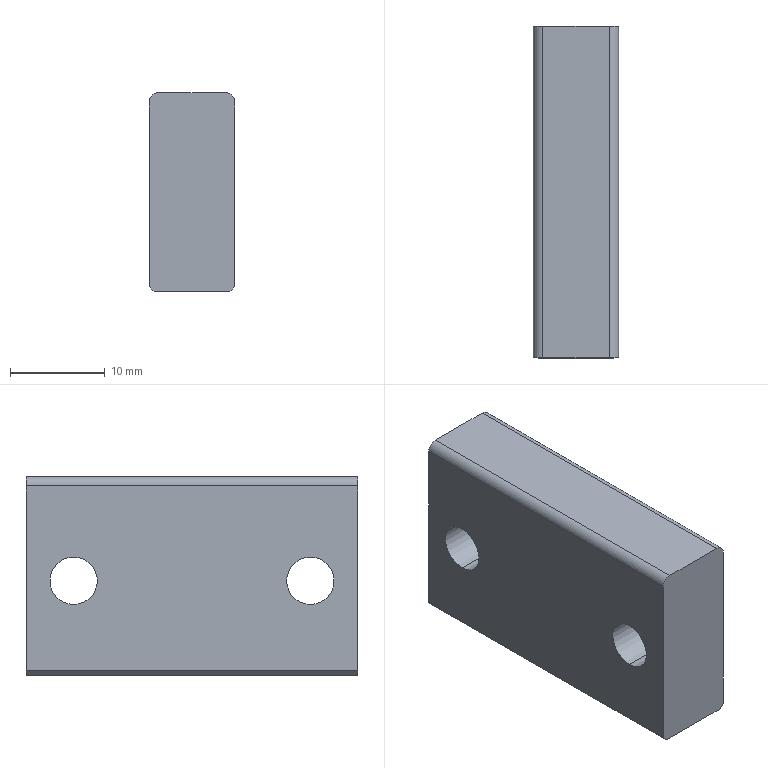Part | SolidWorks | features HoleWzd 2, Chamfer 1, Extrusion 1, Fillet 1 | 1 solid | 22 faces | box 9 x 35 x 21 mm | volume 5976 mm3 | cylinder 10 | plane 8 | cone 4 | commonest cylinder face diameters 3.3 x4 5 x4 2 x2
STEP:
#1=CARTESIAN_POINT('',(6.15,4.5,15.));
#2=VERTEX_POINT('',#1);
#3=CARTESIAN_POINT('',(2.85,4.5,15.));
#4=VERTEX_POINT('',#3);
#5=CARTESIAN_POINT('',(4.5,4.5,15.));
#6=DIRECTION('',(0.,0.,-1.));
#7=DIRECTION('',(-1.,0.,0.));
#8=AXIS2_PLACEMENT_3D('',#5,#6,#7);
#9=CIRCLE('',#8,1.65);
#10=EDGE_CURVE('',#2,#4,#9,.T.);
#11=ORIENTED_EDGE('',*,*,#10,.F.);
#12=CARTESIAN_POINT('',(6.15,4.5,0.));
#13=VERTEX_POINT('',#12);
#14=CARTESIAN_POINT('',(6.15,4.5,0.));
#15=DIRECTION('',(0.,0.,-1.));
#16=VECTOR('',#15,1000.);
#17=LINE('',#14,#16);
#18=EDGE_CURVE('',#2,#13,#17,.T.);
#19=ORIENTED_EDGE('',*,*,#18,.T.);
#20=CARTESIAN_POINT('',(2.85,4.5,0.));
#21=VERTEX_POINT('',#20);
#22=CARTESIAN_POINT('',(4.5,4.5,0.));
#23=DIRECTION('',(0.,0.,-1.));
#24=DIRECTION('',(-1.,0.,0.));
#25=AXIS2_PLACEMENT_3D('',#22,#23,#24);
#26=CIRCLE('',#25,1.65);
#27=EDGE_CURVE('',#13,#21,#26,.T.);
#28=ORIENTED_EDGE('',*,*,#27,.T.);
#29=CARTESIAN_POINT('',(2.85,4.5,0.));
#30=DIRECTION('',(0.,0.,-1.));
#31=VECTOR('',#30,1000.);
#32=LINE('',#29,#31);
#33=EDGE_CURVE('',#4,#21,#32,.T.);
#34=ORIENTED_EDGE('',*,*,#33,.F.);
#35=EDGE_LOOP('',(#11,#19,#28,#34));
#36=FACE_OUTER_BOUND('',#35,.T.);
#37=CARTESIAN_POINT('',(4.5,4.5,0.));
#38=DIRECTION('',(0.,0.,-1.));
#39=DIRECTION('',(-1.,0.,0.));
#40=AXIS2_PLACEMENT_3D('',#37,#38,#39);
#41=CYLINDRICAL_SURFACE('',#40,1.65);
#42=ADVANCED_FACE('',(#36),#41,.F.);
#43=CARTESIAN_POINT('',(4.5,4.5,15.991));
#44=VERTEX_POINT('',#43);
#45=CARTESIAN_POINT('',(2.85,4.5,15.));
#46=DIRECTION('',(-0.8572,0.,-0.515));
#47=VECTOR('',#46,1000.);
#48=LINE('',#45,#47);
#49=EDGE_CURVE('',#44,#4,#48,.T.);
#50=ORIENTED_EDGE('',*,*,#49,.F.);
#51=CARTESIAN_POINT('',(6.15,4.5,15.));
#52=DIRECTION('',(0.8572,0.,-0.515));
#53=VECTOR('',#52,1000.);
#54=LINE('',#51,#53);
#55=EDGE_CURVE('',#44,#2,#54,.T.);
#56=ORIENTED_EDGE('',*,*,#55,.T.);
#57=ORIENTED_EDGE('',*,*,#10,.T.);
#58=EDGE_LOOP('',(#50,#56,#57));
#59=FACE_OUTER_BOUND('',#58,.T.);
#60=CARTESIAN_POINT('',(4.5,4.5,15.));
#61=DIRECTION('',(0.,0.,-1.));
#62=DIRECTION('',(-1.,0.,0.));
#63=AXIS2_PLACEMENT_3D('',#60,#61,#62);
#64=CONICAL_SURFACE('',#63,1.65,1.03);
#65=ADVANCED_FACE('',(#59),#64,.F.);
#66=CARTESIAN_POINT('',(6.15,-4.5,15.));
#67=VERTEX_POINT('',#66);
#68=CARTESIAN_POINT('',(2.85,-4.5,15.));
#69=VERTEX_POINT('',#68);
#70=CARTESIAN_POINT('',(4.5,-4.5,15.));
#71=DIRECTION('',(0.,0.,-1.));
#72=DIRECTION('',(-1.,0.,0.));
#73=AXIS2_PLACEMENT_3D('',#70,#71,#72);
#74=CIRCLE('',#73,1.65);
#75=EDGE_CURVE('',#67,#69,#74,.T.);
#76=ORIENTED_EDGE('',*,*,#75,.F.);
#77=CARTESIAN_POINT('',(6.15,-4.5,0.));
#78=VERTEX_POINT('',#77);
#79=CARTESIAN_POINT('',(6.15,-4.5,0.));
#80=DIRECTION('',(0.,0.,-1.));
#81=VECTOR('',#80,1000.);
#82=LINE('',#79,#81);
#83=EDGE_CURVE('',#67,#78,#82,.T.);
#84=ORIENTED_EDGE('',*,*,#83,.T.);
#85=CARTESIAN_POINT('',(2.85,-4.5,0.));
#86=VERTEX_POINT('',#85);
#87=CARTESIAN_POINT('',(4.5,-4.5,0.));
#88=DIRECTION('',(0.,0.,-1.));
#89=DIRECTION('',(-1.,0.,0.));
#90=AXIS2_PLACEMENT_3D('',#87,#88,#89);
#91=CIRCLE('',#90,1.65);
#92=EDGE_CURVE('',#78,#86,#91,.T.);
#93=ORIENTED_EDGE('',*,*,#92,.T.);
#94=CARTESIAN_POINT('',(2.85,-4.5,0.));
#95=DIRECTION('',(0.,0.,-1.));
#96=VECTOR('',#95,1000.);
#97=LINE('',#94,#96);
#98=EDGE_CURVE('',#69,#86,#97,.T.);
#99=ORIENTED_EDGE('',*,*,#98,.F.);
#100=EDGE_LOOP('',(#76,#84,#93,#99));
#101=FACE_OUTER_BOUND('',#100,.T.);
#102=CARTESIAN_POINT('',(4.5,-4.5,0.));
#103=DIRECTION('',(0.,0.,-1.));
#104=DIRECTION('',(-1.,0.,0.));
#105=AXIS2_PLACEMENT_3D('',#102,#103,#104);
#106=CYLINDRICAL_SURFACE('',#105,1.65);
#107=ADVANCED_FACE('',(#101),#106,.F.);
#108=CARTESIAN_POINT('',(4.5,-4.5,15.991));
#109=VERTEX_POINT('',#108);
#110=CARTESIAN_POINT('',(2.85,-4.5,15.));
#111=DIRECTION('',(-0.8572,0.,-0.515));
#112=VECTOR('',#111,1000.);
#113=LINE('',#110,#112);
#114=EDGE_CURVE('',#109,#69,#113,.T.);
#115=ORIENTED_EDGE('',*,*,#114,.F.);
#116=CARTESIAN_POINT('',(6.15,-4.5,15.));
#117=DIRECTION('',(0.8572,0.,-0.515));
#118=VECTOR('',#117,1000.);
#119=LINE('',#116,#118);
#120=EDGE_CURVE('',#109,#67,#119,.T.);
#121=ORIENTED_EDGE('',*,*,#120,.T.);
#122=ORIENTED_EDGE('',*,*,#75,.T.);
#123=EDGE_LOOP('',(#115,#121,#122));
#124=FACE_OUTER_BOUND('',#123,.T.);
#125=CARTESIAN_POINT('',(4.5,-4.5,15.));
#126=DIRECTION('',(0.,0.,-1.));
#127=DIRECTION('',(-1.,0.,0.));
#128=AXIS2_PLACEMENT_3D('',#125,#126,#127);
#129=CONICAL_SURFACE('',#128,1.65,1.03);
#130=ADVANCED_FACE('',(#124),#129,.F.);
#131=CARTESIAN_POINT('',(0.,12.5,12.5));
#132=VERTEX_POINT('',#131);
#133=CARTESIAN_POINT('',(0.,12.5,7.5));
#134=VERTEX_POINT('',#133);
#135=CARTESIAN_POINT('',(0.,12.5,10.));
#136=DIRECTION('',(1.,0.,0.));
#137=DIRECTION('',(0.,0.,-1.));
#138=AXIS2_PLACEMENT_3D('',#135,#136,#137);
#139=CIRCLE('',#138,2.5);
#140=EDGE_CURVE('',#132,#134,#139,.T.);
#141=ORIENTED_EDGE('',*,*,#140,.F.);
#142=CARTESIAN_POINT('',(9.,12.5,12.5));
#143=VERTEX_POINT('',#142);
#144=CARTESIAN_POINT('',(9.,12.5,12.5));
#145=DIRECTION('',(1.,0.,0.));
#146=VECTOR('',#145,1000.);
#147=LINE('',#144,#146);
#148=EDGE_CURVE('',#132,#143,#147,.T.);
#149=ORIENTED_EDGE('',*,*,#148,.T.);
#150=CARTESIAN_POINT('',(9.,12.5,7.5));
#151=VERTEX_POINT('',#150);
#152=CARTESIAN_POINT('',(9.,12.5,10.));
#153=DIRECTION('',(1.,0.,0.));
#154=DIRECTION('',(0.,0.,-1.));
#155=AXIS2_PLACEMENT_3D('',#152,#153,#154);
#156=CIRCLE('',#155,2.5);
#157=EDGE_CURVE('',#143,#151,#156,.T.);
#158=ORIENTED_EDGE('',*,*,#157,.T.);
#159=CARTESIAN_POINT('',(9.,12.5,7.5));
#160=DIRECTION('',(1.,0.,0.));
#161=VECTOR('',#160,1000.);
#162=LINE('',#159,#161);
#163=EDGE_CURVE('',#134,#151,#162,.T.);
#164=ORIENTED_EDGE('',*,*,#163,.F.);
#165=EDGE_LOOP('',(#141,#149,#158,#164));
#166=FACE_OUTER_BOUND('',#165,.T.);
#167=CARTESIAN_POINT('',(9.,12.5,10.));
#168=DIRECTION('',(1.,0.,0.));
#169=DIRECTION('',(0.,0.,-1.));
#170=AXIS2_PLACEMENT_3D('',#167,#168,#169);
#171=CYLINDRICAL_SURFACE('',#170,2.5);
#172=ADVANCED_FACE('',(#166),#171,.F.);
#173=CARTESIAN_POINT('',(0.,-12.5,12.5));
#174=VERTEX_POINT('',#173);
#175=CARTESIAN_POINT('',(0.,-12.5,7.5));
#176=VERTEX_POINT('',#175);
#177=CARTESIAN_POINT('',(0.,-12.5,10.));
#178=DIRECTION('',(1.,0.,0.));
#179=DIRECTION('',(0.,0.,-1.));
#180=AXIS2_PLACEMENT_3D('',#177,#178,#179);
#181=CIRCLE('',#180,2.5);
#182=EDGE_CURVE('',#174,#176,#181,.T.);
#183=ORIENTED_EDGE('',*,*,#182,.F.);
#184=CARTESIAN_POINT('',(9.,-12.5,12.5));
#185=VERTEX_POINT('',#184);
#186=CARTESIAN_POINT('',(9.,-12.5,12.5));
#187=DIRECTION('',(1.,0.,0.));
#188=VECTOR('',#187,1000.);
#189=LINE('',#186,#188);
#190=EDGE_CURVE('',#174,#185,#189,.T.);
#191=ORIENTED_EDGE('',*,*,#190,.T.);
#192=CARTESIAN_POINT('',(9.,-12.5,7.5));
#193=VERTEX_POINT('',#192);
#194=CARTESIAN_POINT('',(9.,-12.5,10.));
#195=DIRECTION('',(1.,0.,0.));
#196=DIRECTION('',(0.,0.,-1.));
#197=AXIS2_PLACEMENT_3D('',#194,#195,#196);
#198=CIRCLE('',#197,2.5);
#199=EDGE_CURVE('',#185,#193,#198,.T.);
#200=ORIENTED_EDGE('',*,*,#199,.T.);
#201=CARTESIAN_POINT('',(9.,-12.5,7.5));
#202=DIRECTION('',(1.,0.,0.));
#203=VECTOR('',#202,1000.);
#204=LINE('',#201,#203);
#205=EDGE_CURVE('',#176,#193,#204,.T.);
#206=ORIENTED_EDGE('',*,*,#205,.F.);
#207=EDGE_LOOP('',(#183,#191,#200,#206));
#208=FACE_OUTER_BOUND('',#207,.T.);
#209=CARTESIAN_POINT('',(9.,-12.5,10.));
#210=DIRECTION('',(1.,0.,0.));
#211=DIRECTION('',(0.,0.,-1.));
#212=AXIS2_PLACEMENT_3D('',#209,#210,#211);
#213=CYLINDRICAL_SURFACE('',#212,2.5);
#214=ADVANCED_FACE('',(#208),#213,.F.);
#215=CARTESIAN_POINT('',(0.,12.5,10.));
#216=DIRECTION('',(1.,0.,0.));
#217=DIRECTION('',(0.,0.,-1.));
#218=AXIS2_PLACEMENT_3D('',#215,#216,#217);
#219=CIRCLE('',#218,2.5);
#220=EDGE_CURVE('',#134,#132,#219,.T.);
#221=ORIENTED_EDGE('',*,*,#220,.T.);
#222=ORIENTED_EDGE('',*,*,#140,.T.);
#223=EDGE_LOOP('',(#221,#222));
#224=FACE_BOUND('',#223,.T.);
#225=CARTESIAN_POINT('',(0.,-12.5,10.));
#226=DIRECTION('',(1.,0.,0.));
#227=DIRECTION('',(0.,0.,-1.));
#228=AXIS2_PLACEMENT_3D('',#225,#226,#227);
#229=CIRCLE('',#228,2.5);
#230=EDGE_CURVE('',#176,#174,#229,.T.);
#231=ORIENTED_EDGE('',*,*,#230,.T.);
#232=ORIENTED_EDGE('',*,*,#182,.T.);
#233=EDGE_LOOP('',(#231,#232));
#234=FACE_BOUND('',#233,.T.);
#235=CARTESIAN_POINT('',(0.,17.5,20.));
#236=VERTEX_POINT('',#235);
#237=CARTESIAN_POINT('',(0.,17.5,0.5));
#238=VERTEX_POINT('',#237);
#239=CARTESIAN_POINT('',(0.,17.5,21.));
#240=DIRECTION('',(0.,0.,-1.));
#241=VECTOR('',#240,1000.);
#242=LINE('',#239,#241);
#243=EDGE_CURVE('',#236,#238,#242,.T.);
#244=ORIENTED_EDGE('',*,*,#243,.T.);
#245=CARTESIAN_POINT('',(0.,-17.5,0.5));
#246=VERTEX_POINT('',#245);
#247=CARTESIAN_POINT('',(0.,17.5,0.5));
#248=DIRECTION('',(0.,-1.,0.));
#249=VECTOR('',#248,1000.);
#250=LINE('',#247,#249);
#251=EDGE_CURVE('',#238,#246,#250,.T.);
#252=ORIENTED_EDGE('',*,*,#251,.T.);
#253=CARTESIAN_POINT('',(0.,-17.5,20.));
#254=VERTEX_POINT('',#253);
#255=CARTESIAN_POINT('',(0.,-17.5,21.));
#256=DIRECTION('',(0.,0.,-1.));
#257=VECTOR('',#256,1000.);
#258=LINE('',#255,#257);
#259=EDGE_CURVE('',#254,#246,#258,.T.);
#260=ORIENTED_EDGE('',*,*,#259,.F.);
#261=CARTESIAN_POINT('',(0.,17.5,20.));
#262=DIRECTION('',(0.,1.,0.));
#263=VECTOR('',#262,1000.);
#264=LINE('',#261,#263);
#265=EDGE_CURVE('',#254,#236,#264,.T.);
#266=ORIENTED_EDGE('',*,*,#265,.T.);
#267=EDGE_LOOP('',(#244,#252,#260,#266));
#268=FACE_OUTER_BOUND('',#267,.T.);
#269=CARTESIAN_POINT('',(0.,17.5,21.));
#270=DIRECTION('',(1.,0.,0.));
#271=DIRECTION('',(0.,0.,-1.));
#272=AXIS2_PLACEMENT_3D('',#269,#270,#271);
#273=PLANE('',#272);
#274=ADVANCED_FACE('',(#224,#234,#268),#273,.F.);
#275=ORIENTED_EDGE('',*,*,#259,.T.);
#276=CARTESIAN_POINT('',(0.5,-17.5,0.));
#277=VERTEX_POINT('',#276);
#278=CARTESIAN_POINT('',(0.,-17.5,0.5));
#279=DIRECTION('',(0.7071,0.,-0.7071));
#280=VECTOR('',#279,1000.);
#281=LINE('',#278,#280);
#282=EDGE_CURVE('',#246,#277,#281,.T.);
#283=ORIENTED_EDGE('',*,*,#282,.T.);
#284=CARTESIAN_POINT('',(8.5,-17.5,0.));
#285=VERTEX_POINT('',#284);
#286=CARTESIAN_POINT('',(0.,-17.5,0.));
#287=DIRECTION('',(1.,0.,0.));
#288=VECTOR('',#287,1000.);
#289=LINE('',#286,#288);
#290=EDGE_CURVE('',#277,#285,#289,.T.);
#291=ORIENTED_EDGE('',*,*,#290,.T.);
#292=CARTESIAN_POINT('',(9.,-17.5,0.5));
#293=VERTEX_POINT('',#292);
#294=CARTESIAN_POINT('',(9.,-17.5,0.5));
#295=DIRECTION('',(0.7071,0.,0.7071));
#296=VECTOR('',#295,1000.);
#297=LINE('',#294,#296);
#298=EDGE_CURVE('',#285,#293,#297,.T.);
#299=ORIENTED_EDGE('',*,*,#298,.T.);
#300=CARTESIAN_POINT('',(9.,-17.5,20.));
#301=VERTEX_POINT('',#300);
#302=CARTESIAN_POINT('',(9.,-17.5,21.));
#303=DIRECTION('',(0.,0.,-1.));
#304=VECTOR('',#303,1000.);
#305=LINE('',#302,#304);
#306=EDGE_CURVE('',#301,#293,#305,.T.);
#307=ORIENTED_EDGE('',*,*,#306,.F.);
#308=CARTESIAN_POINT('',(8.,-17.5,21.));
#309=VERTEX_POINT('',#308);
#310=CARTESIAN_POINT('',(8.,-17.5,20.));
#311=DIRECTION('',(0.,-1.,0.));
#312=DIRECTION('',(0.,0.,1.));
#313=AXIS2_PLACEMENT_3D('',#310,#311,#312);
#314=CIRCLE('',#313,1.);
#315=EDGE_CURVE('',#301,#309,#314,.T.);
#316=ORIENTED_EDGE('',*,*,#315,.T.);
#317=CARTESIAN_POINT('',(1.,-17.5,21.));
#318=VERTEX_POINT('',#317);
#319=CARTESIAN_POINT('',(0.,-17.5,21.));
#320=DIRECTION('',(1.,0.,0.));
#321=VECTOR('',#320,1000.);
#322=LINE('',#319,#321);
#323=EDGE_CURVE('',#318,#309,#322,.T.);
#324=ORIENTED_EDGE('',*,*,#323,.F.);
#325=CARTESIAN_POINT('',(1.,-17.5,20.));
#326=DIRECTION('',(0.,-1.,0.));
#327=DIRECTION('',(0.,0.,1.));
#328=AXIS2_PLACEMENT_3D('',#325,#326,#327);
#329=CIRCLE('',#328,1.);
#330=EDGE_CURVE('',#318,#254,#329,.T.);
#331=ORIENTED_EDGE('',*,*,#330,.T.);
#332=EDGE_LOOP('',(#275,#283,#291,#299,#307,#316,#324,#331));
#333=FACE_OUTER_BOUND('',#332,.T.);
#334=CARTESIAN_POINT('',(0.,-17.5,21.));
#335=DIRECTION('',(0.,1.,0.));
#336=DIRECTION('',(0.,0.,1.));
#337=AXIS2_PLACEMENT_3D('',#334,#335,#336);
#338=PLANE('',#337);
#339=ADVANCED_FACE('',(#333),#338,.F.);
#340=CARTESIAN_POINT('',(9.,12.5,10.));
#341=DIRECTION('',(1.,0.,0.));
#342=DIRECTION('',(0.,0.,-1.));
#343=AXIS2_PLACEMENT_3D('',#340,#341,#342);
#344=CIRCLE('',#343,2.5);
#345=EDGE_CURVE('',#151,#143,#344,.T.);
#346=ORIENTED_EDGE('',*,*,#345,.F.);
#347=ORIENTED_EDGE('',*,*,#157,.F.);
#348=EDGE_LOOP('',(#346,#347));
#349=FACE_BOUND('',#348,.T.);
#350=CARTESIAN_POINT('',(9.,-12.5,10.));
#351=DIRECTION('',(1.,0.,0.));
#352=DIRECTION('',(0.,0.,-1.));
#353=AXIS2_PLACEMENT_3D('',#350,#351,#352);
#354=CIRCLE('',#353,2.5);
#355=EDGE_CURVE('',#193,#185,#354,.T.);
#356=ORIENTED_EDGE('',*,*,#355,.F.);
#357=ORIENTED_EDGE('',*,*,#199,.F.);
#358=EDGE_LOOP('',(#356,#357));
#359=FACE_BOUND('',#358,.T.);
#360=ORIENTED_EDGE('',*,*,#306,.T.);
#361=CARTESIAN_POINT('',(9.,17.5,0.5));
#362=VERTEX_POINT('',#361);
#363=CARTESIAN_POINT('',(9.,17.5,0.5));
#364=DIRECTION('',(0.,1.,0.));
#365=VECTOR('',#364,1000.);
#366=LINE('',#363,#365);
#367=EDGE_CURVE('',#293,#362,#366,.T.);
#368=ORIENTED_EDGE('',*,*,#367,.T.);
#369=CARTESIAN_POINT('',(9.,17.5,20.));
#370=VERTEX_POINT('',#369);
#371=CARTESIAN_POINT('',(9.,17.5,21.));
#372=DIRECTION('',(0.,0.,-1.));
#373=VECTOR('',#372,1000.);
#374=LINE('',#371,#373);
#375=EDGE_CURVE('',#370,#362,#374,.T.);
#376=ORIENTED_EDGE('',*,*,#375,.F.);
#377=CARTESIAN_POINT('',(9.,-17.5,20.));
#378=DIRECTION('',(0.,-1.,0.));
#379=VECTOR('',#378,1000.);
#380=LINE('',#377,#379);
#381=EDGE_CURVE('',#370,#301,#380,.T.);
#382=ORIENTED_EDGE('',*,*,#381,.T.);
#383=EDGE_LOOP('',(#360,#368,#376,#382));
#384=FACE_OUTER_BOUND('',#383,.T.);
#385=CARTESIAN_POINT('',(9.,17.5,21.));
#386=DIRECTION('',(-1.,0.,0.));
#387=DIRECTION('',(0.,0.,1.));
#388=AXIS2_PLACEMENT_3D('',#385,#386,#387);
#389=PLANE('',#388);
#390=ADVANCED_FACE('',(#349,#359,#384),#389,.F.);
#391=CARTESIAN_POINT('',(8.5,17.5,0.));
#392=VERTEX_POINT('',#391);
#393=CARTESIAN_POINT('',(0.5,17.5,0.));
#394=VERTEX_POINT('',#393);
#395=CARTESIAN_POINT('',(0.,17.5,0.));
#396=DIRECTION('',(-1.,0.,0.));
#397=VECTOR('',#396,1000.);
#398=LINE('',#395,#397);
#399=EDGE_CURVE('',#392,#394,#398,.T.);
#400=ORIENTED_EDGE('',*,*,#399,.T.);
#401=CARTESIAN_POINT('',(0.,17.5,0.5));
#402=DIRECTION('',(-0.7071,0.,0.7071));
#403=VECTOR('',#402,1000.);
#404=LINE('',#401,#403);
#405=EDGE_CURVE('',#394,#238,#404,.T.);
#406=ORIENTED_EDGE('',*,*,#405,.T.);
#407=ORIENTED_EDGE('',*,*,#243,.F.);
#408=CARTESIAN_POINT('',(1.,17.5,21.));
#409=VERTEX_POINT('',#408);
#410=CARTESIAN_POINT('',(1.,17.5,20.));
#411=DIRECTION('',(0.,1.,0.));
#412=DIRECTION('',(0.,0.,-1.));
#413=AXIS2_PLACEMENT_3D('',#410,#411,#412);
#414=CIRCLE('',#413,1.);
#415=EDGE_CURVE('',#236,#409,#414,.T.);
#416=ORIENTED_EDGE('',*,*,#415,.T.);
#417=CARTESIAN_POINT('',(8.,17.5,21.));
#418=VERTEX_POINT('',#417);
#419=CARTESIAN_POINT('',(0.,17.5,21.));
#420=DIRECTION('',(-1.,0.,0.));
#421=VECTOR('',#420,1000.);
#422=LINE('',#419,#421);
#423=EDGE_CURVE('',#418,#409,#422,.T.);
#424=ORIENTED_EDGE('',*,*,#423,.F.);
#425=CARTESIAN_POINT('',(8.,17.5,20.));
#426=DIRECTION('',(0.,1.,0.));
#427=DIRECTION('',(0.,0.,-1.));
#428=AXIS2_PLACEMENT_3D('',#425,#426,#427);
#429=CIRCLE('',#428,1.);
#430=EDGE_CURVE('',#418,#370,#429,.T.);
#431=ORIENTED_EDGE('',*,*,#430,.T.);
#432=ORIENTED_EDGE('',*,*,#375,.T.);
#433=CARTESIAN_POINT('',(9.,17.5,0.5));
#434=DIRECTION('',(-0.7071,0.,-0.7071));
#435=VECTOR('',#434,1000.);
#436=LINE('',#433,#435);
#437=EDGE_CURVE('',#362,#392,#436,.T.);
#438=ORIENTED_EDGE('',*,*,#437,.T.);
#439=EDGE_LOOP('',(#400,#406,#407,#416,#424,#431,#432,#438));
#440=FACE_OUTER_BOUND('',#439,.T.);
#441=CARTESIAN_POINT('',(0.,17.5,21.));
#442=DIRECTION('',(0.,-1.,0.));
#443=DIRECTION('',(0.,0.,-1.));
#444=AXIS2_PLACEMENT_3D('',#441,#442,#443);
#445=PLANE('',#444);
#446=ADVANCED_FACE('',(#440),#445,.F.);
#447=ORIENTED_EDGE('',*,*,#423,.T.);
#448=CARTESIAN_POINT('',(1.,-17.5,21.));
#449=DIRECTION('',(0.,-1.,0.));
#450=VECTOR('',#449,1000.);
#451=LINE('',#448,#450);
#452=EDGE_CURVE('',#409,#318,#451,.T.);
#453=ORIENTED_EDGE('',*,*,#452,.T.);
#454=ORIENTED_EDGE('',*,*,#323,.T.);
#455=CARTESIAN_POINT('',(8.,17.5,21.));
#456=DIRECTION('',(0.,1.,0.));
#457=VECTOR('',#456,1000.);
#458=LINE('',#455,#457);
#459=EDGE_CURVE('',#309,#418,#458,.T.);
#460=ORIENTED_EDGE('',*,*,#459,.T.);
#461=EDGE_LOOP('',(#447,#453,#454,#460));
#462=FACE_OUTER_BOUND('',#461,.T.);
#463=CARTESIAN_POINT('',(0.,-17.5,21.));
#464=DIRECTION('',(0.,0.,1.));
#465=DIRECTION('',(1.,0.,0.));
#466=AXIS2_PLACEMENT_3D('',#463,#464,#465);
#467=PLANE('',#466);
#468=ADVANCED_FACE('',(#462),#467,.T.);
#469=CARTESIAN_POINT('',(4.5,4.5,0.));
#470=DIRECTION('',(0.,0.,-1.));
#471=DIRECTION('',(-1.,0.,0.));
#472=AXIS2_PLACEMENT_3D('',#469,#470,#471);
#473=CIRCLE('',#472,1.65);
#474=EDGE_CURVE('',#21,#13,#473,.T.);
#475=ORIENTED_EDGE('',*,*,#474,.F.);
#476=ORIENTED_EDGE('',*,*,#27,.F.);
#477=EDGE_LOOP('',(#475,#476));
#478=FACE_BOUND('',#477,.T.);
#479=CARTESIAN_POINT('',(4.5,-4.5,0.));
#480=DIRECTION('',(0.,0.,-1.));
#481=DIRECTION('',(-1.,0.,0.));
#482=AXIS2_PLACEMENT_3D('',#479,#480,#481);
#483=CIRCLE('',#482,1.65);
#484=EDGE_CURVE('',#86,#78,#483,.T.);
#485=ORIENTED_EDGE('',*,*,#484,.F.);
#486=ORIENTED_EDGE('',*,*,#92,.F.);
#487=EDGE_LOOP('',(#485,#486));
#488=FACE_BOUND('',#487,.T.);
#489=ORIENTED_EDGE('',*,*,#290,.F.);
#490=CARTESIAN_POINT('',(0.5,-17.5,0.));
#491=DIRECTION('',(0.,1.,0.));
#492=VECTOR('',#491,1000.);
#493=LINE('',#490,#492);
#494=EDGE_CURVE('',#277,#394,#493,.T.);
#495=ORIENTED_EDGE('',*,*,#494,.T.);
#496=ORIENTED_EDGE('',*,*,#399,.F.);
#497=CARTESIAN_POINT('',(8.5,-17.5,0.));
#498=DIRECTION('',(0.,-1.,0.));
#499=VECTOR('',#498,1000.);
#500=LINE('',#497,#499);
#501=EDGE_CURVE('',#392,#285,#500,.T.);
#502=ORIENTED_EDGE('',*,*,#501,.T.);
#503=EDGE_LOOP('',(#489,#495,#496,#502));
#504=FACE_OUTER_BOUND('',#503,.T.);
#505=CARTESIAN_POINT('',(0.,-17.5,0.));
#506=DIRECTION('',(0.,0.,1.));
#507=DIRECTION('',(1.,0.,0.));
#508=AXIS2_PLACEMENT_3D('',#505,#506,#507);
#509=PLANE('',#508);
#510=ADVANCED_FACE('',(#478,#488,#504),#509,.F.);
#511=ORIENTED_EDGE('',*,*,#190,.F.);
#512=ORIENTED_EDGE('',*,*,#230,.F.);
#513=ORIENTED_EDGE('',*,*,#205,.T.);
#514=ORIENTED_EDGE('',*,*,#355,.T.);
#515=EDGE_LOOP('',(#511,#512,#513,#514));
#516=FACE_OUTER_BOUND('',#515,.T.);
#517=CARTESIAN_POINT('',(9.,-12.5,10.));
#518=DIRECTION('',(1.,0.,0.));
#519=DIRECTION('',(0.,0.,-1.));
#520=AXIS2_PLACEMENT_3D('',#517,#518,#519);
#521=CYLINDRICAL_SURFACE('',#520,2.5);
#522=ADVANCED_FACE('',(#516),#521,.F.);
#523=ORIENTED_EDGE('',*,*,#148,.F.);
#524=ORIENTED_EDGE('',*,*,#220,.F.);
#525=ORIENTED_EDGE('',*,*,#163,.T.);
#526=ORIENTED_EDGE('',*,*,#345,.T.);
#527=EDGE_LOOP('',(#523,#524,#525,#526));
#528=FACE_OUTER_BOUND('',#527,.T.);
#529=CARTESIAN_POINT('',(9.,12.5,10.));
#530=DIRECTION('',(1.,0.,0.));
#531=DIRECTION('',(0.,0.,-1.));
#532=AXIS2_PLACEMENT_3D('',#529,#530,#531);
#533=CYLINDRICAL_SURFACE('',#532,2.5);
#534=ADVANCED_FACE('',(#528),#533,.F.);
#535=ORIENTED_EDGE('',*,*,#120,.F.);
#536=ORIENTED_EDGE('',*,*,#114,.T.);
#537=CARTESIAN_POINT('',(4.5,-4.5,15.));
#538=DIRECTION('',(0.,0.,-1.));
#539=DIRECTION('',(-1.,0.,0.));
#540=AXIS2_PLACEMENT_3D('',#537,#538,#539);
#541=CIRCLE('',#540,1.65);
#542=EDGE_CURVE('',#69,#67,#541,.T.);
#543=ORIENTED_EDGE('',*,*,#542,.T.);
#544=EDGE_LOOP('',(#535,#536,#543));
#545=FACE_OUTER_BOUND('',#544,.T.);
#546=CARTESIAN_POINT('',(4.5,-4.5,15.));
#547=DIRECTION('',(0.,0.,-1.));
#548=DIRECTION('',(-1.,0.,0.));
#549=AXIS2_PLACEMENT_3D('',#546,#547,#548);
#550=CONICAL_SURFACE('',#549,1.65,1.03);
#551=ADVANCED_FACE('',(#545),#550,.F.);
#552=ORIENTED_EDGE('',*,*,#83,.F.);
#553=ORIENTED_EDGE('',*,*,#542,.F.);
#554=ORIENTED_EDGE('',*,*,#98,.T.);
#555=ORIENTED_EDGE('',*,*,#484,.T.);
#556=EDGE_LOOP('',(#552,#553,#554,#555));
#557=FACE_OUTER_BOUND('',#556,.T.);
#558=CARTESIAN_POINT('',(4.5,-4.5,0.));
#559=DIRECTION('',(0.,0.,-1.));
#560=DIRECTION('',(-1.,0.,0.));
#561=AXIS2_PLACEMENT_3D('',#558,#559,#560);
#562=CYLINDRICAL_SURFACE('',#561,1.65);
#563=ADVANCED_FACE('',(#557),#562,.F.);
#564=ORIENTED_EDGE('',*,*,#55,.F.);
#565=ORIENTED_EDGE('',*,*,#49,.T.);
#566=CARTESIAN_POINT('',(4.5,4.5,15.));
#567=DIRECTION('',(0.,0.,-1.));
#568=DIRECTION('',(-1.,0.,0.));
#569=AXIS2_PLACEMENT_3D('',#566,#567,#568);
#570=CIRCLE('',#569,1.65);
#571=EDGE_CURVE('',#4,#2,#570,.T.);
#572=ORIENTED_EDGE('',*,*,#571,.T.);
#573=EDGE_LOOP('',(#564,#565,#572));
#574=FACE_OUTER_BOUND('',#573,.T.);
#575=CARTESIAN_POINT('',(4.5,4.5,15.));
#576=DIRECTION('',(0.,0.,-1.));
#577=DIRECTION('',(-1.,0.,0.));
#578=AXIS2_PLACEMENT_3D('',#575,#576,#577);
#579=CONICAL_SURFACE('',#578,1.65,1.03);
#580=ADVANCED_FACE('',(#574),#579,.F.);
#581=ORIENTED_EDGE('',*,*,#18,.F.);
#582=ORIENTED_EDGE('',*,*,#571,.F.);
#583=ORIENTED_EDGE('',*,*,#33,.T.);
#584=ORIENTED_EDGE('',*,*,#474,.T.);
#585=EDGE_LOOP('',(#581,#582,#583,#584));
#586=FACE_OUTER_BOUND('',#585,.T.);
#587=CARTESIAN_POINT('',(4.5,4.5,0.));
#588=DIRECTION('',(0.,0.,-1.));
#589=DIRECTION('',(-1.,0.,0.));
#590=AXIS2_PLACEMENT_3D('',#587,#588,#589);
#591=CYLINDRICAL_SURFACE('',#590,1.65);
#592=ADVANCED_FACE('',(#586),#591,.F.);
#593=ORIENTED_EDGE('',*,*,#415,.F.);
#594=ORIENTED_EDGE('',*,*,#265,.F.);
#595=ORIENTED_EDGE('',*,*,#330,.F.);
#596=ORIENTED_EDGE('',*,*,#452,.F.);
#597=EDGE_LOOP('',(#593,#594,#595,#596));
#598=FACE_OUTER_BOUND('',#597,.T.);
#599=CARTESIAN_POINT('',(1.,-17.5,20.));
#600=DIRECTION('',(0.,1.,0.));
#601=DIRECTION('',(0.,0.,1.));
#602=AXIS2_PLACEMENT_3D('',#599,#600,#601);
#603=CYLINDRICAL_SURFACE('',#602,1.);
#604=ADVANCED_FACE('',(#598),#603,.T.);
#605=ORIENTED_EDGE('',*,*,#315,.F.);
#606=ORIENTED_EDGE('',*,*,#381,.F.);
#607=ORIENTED_EDGE('',*,*,#430,.F.);
#608=ORIENTED_EDGE('',*,*,#459,.F.);
#609=EDGE_LOOP('',(#605,#606,#607,#608));
#610=FACE_OUTER_BOUND('',#609,.T.);
#611=CARTESIAN_POINT('',(8.,-17.5,20.));
#612=DIRECTION('',(0.,-1.,0.));
#613=DIRECTION('',(0.,0.,-1.));
#614=AXIS2_PLACEMENT_3D('',#611,#612,#613);
#615=CYLINDRICAL_SURFACE('',#614,1.);
#616=ADVANCED_FACE('',(#610),#615,.T.);
#617=ORIENTED_EDGE('',*,*,#405,.F.);
#618=ORIENTED_EDGE('',*,*,#494,.F.);
#619=ORIENTED_EDGE('',*,*,#282,.F.);
#620=ORIENTED_EDGE('',*,*,#251,.F.);
#621=EDGE_LOOP('',(#617,#618,#619,#620));
#622=FACE_OUTER_BOUND('',#621,.T.);
#623=CARTESIAN_POINT('',(0.,17.5,0.5));
#624=DIRECTION('',(0.7071,0.,0.7071));
#625=DIRECTION('',(0.,-1.,0.));
#626=AXIS2_PLACEMENT_3D('',#623,#624,#625);
#627=PLANE('',#626);
#628=ADVANCED_FACE('',(#622),#627,.F.);
#629=ORIENTED_EDGE('',*,*,#298,.F.);
#630=ORIENTED_EDGE('',*,*,#501,.F.);
#631=ORIENTED_EDGE('',*,*,#437,.F.);
#632=ORIENTED_EDGE('',*,*,#367,.F.);
#633=EDGE_LOOP('',(#629,#630,#631,#632));
#634=FACE_OUTER_BOUND('',#633,.T.);
#635=CARTESIAN_POINT('',(9.,17.5,0.5));
#636=DIRECTION('',(-0.7071,0.,0.7071));
#637=DIRECTION('',(0.,1.,0.));
#638=AXIS2_PLACEMENT_3D('',#635,#636,#637);
#639=PLANE('',#638);
#640=ADVANCED_FACE('',(#634),#639,.F.);
#641=CLOSED_SHELL('',(#42,#65,#107,#130,#172,#214,#274,#339,#390,#446,#468,#510,#522,#534,#551,#563,#580,#592,#604,#616,#628,#640));
#642=MANIFOLD_SOLID_BREP('',#641);
#643=CARTESIAN_POINT('',(0.,0.,0.));
#644=DIRECTION('',(0.,0.,1.));
#645=DIRECTION('',(1.,0.,0.));
#646=AXIS2_PLACEMENT_3D('',#643,#644,#645);
#647=(LENGTH_UNIT()NAMED_UNIT(*)SI_UNIT(.MILLI.,.METRE.));
#648=UNCERTAINTY_MEASURE_WITH_UNIT(LENGTH_MEASURE(0.00001),#647,'','');
#649=(NAMED_UNIT(*)PLANE_ANGLE_UNIT()SI_UNIT($,.RADIAN.));
#650=(NAMED_UNIT(*)SI_UNIT($,.STERADIAN.)SOLID_ANGLE_UNIT());
#651=(GEOMETRIC_REPRESENTATION_CONTEXT(3)GLOBAL_UNCERTAINTY_ASSIGNED_CONTEXT((#648))GLOBAL_UNIT_ASSIGNED_CONTEXT((#647,#649,#650))REPRESENTATION_CONTEXT('',''));
#652=ADVANCED_BREP_SHAPE_REPRESENTATION('',(#642,#646),#651);